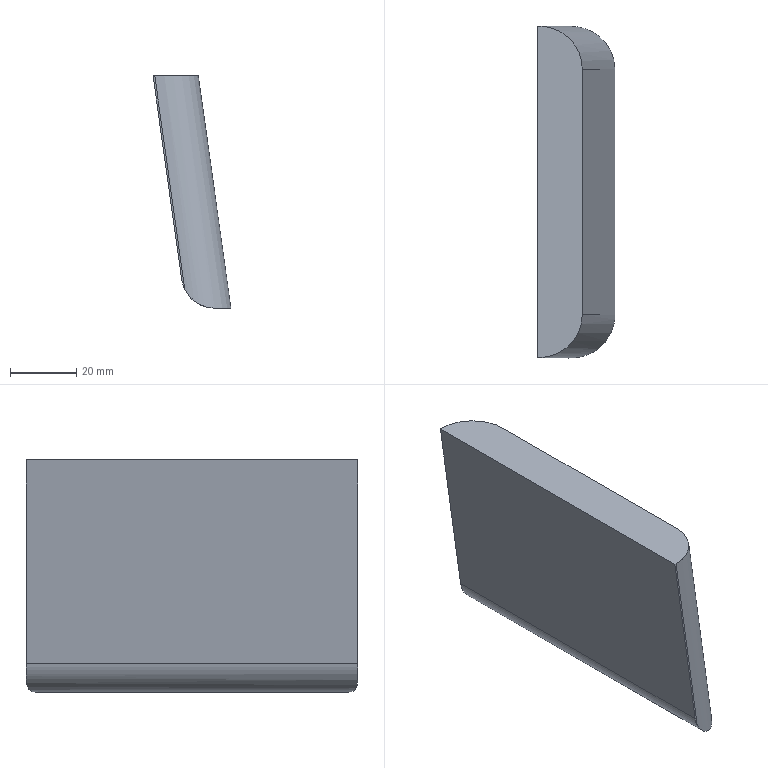Part | STEP file | solid 117 | 1 solid | 9 faces | box 23.471 x 100 x 70 mm | volume 88768 mm3 | plane 6 | cylinder 3 | commonest cylinder face diameters 26 x2 20 x1